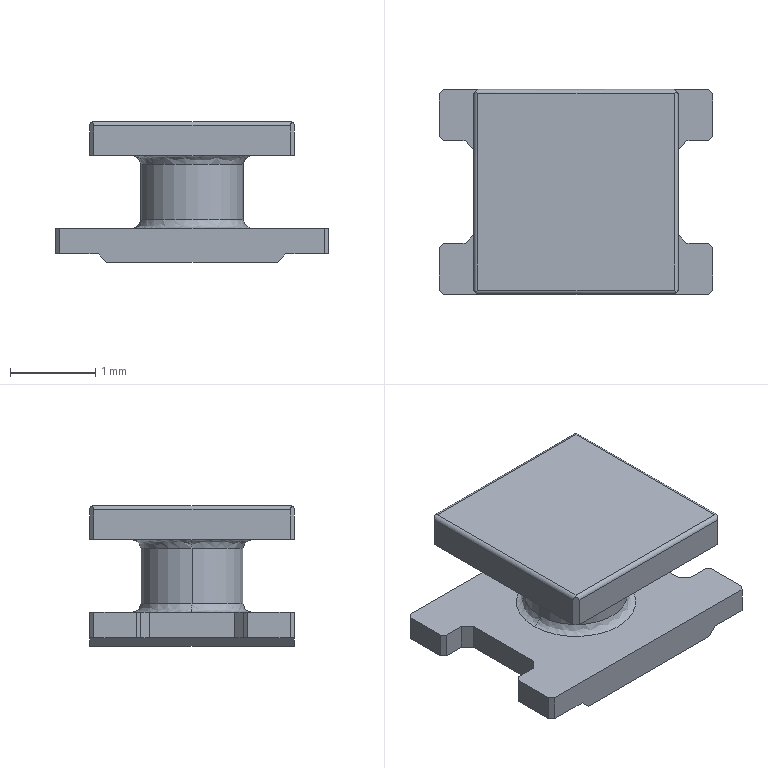Part | SolidWorks | features BaseBody 1 | 1 solid | 50 faces | box 3.2 x 2.4 x 1.65 mm | volume 5.798 mm3 | plane 40 | cylinder 6 | spline 4 | commonest cylinder face diameters 0.1 x4 1.2 x2